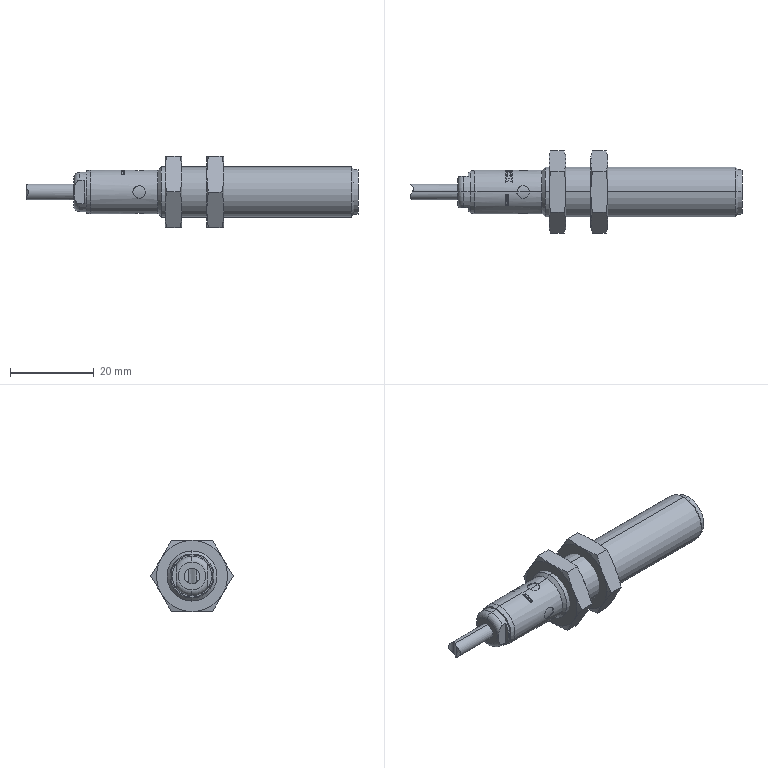Part | SolidWorks | 3 solids | 186 faces | box 79.369 x 19.63 x 17 mm | volume 8383 mm3 | plane 90 | cylinder 35 | cone 34 | spline 25 | torus 2 | commonest cylinder face diameters 10.48 x9 3 x8 10 x5 10.92 x4 3.7 x2 9.4 x2